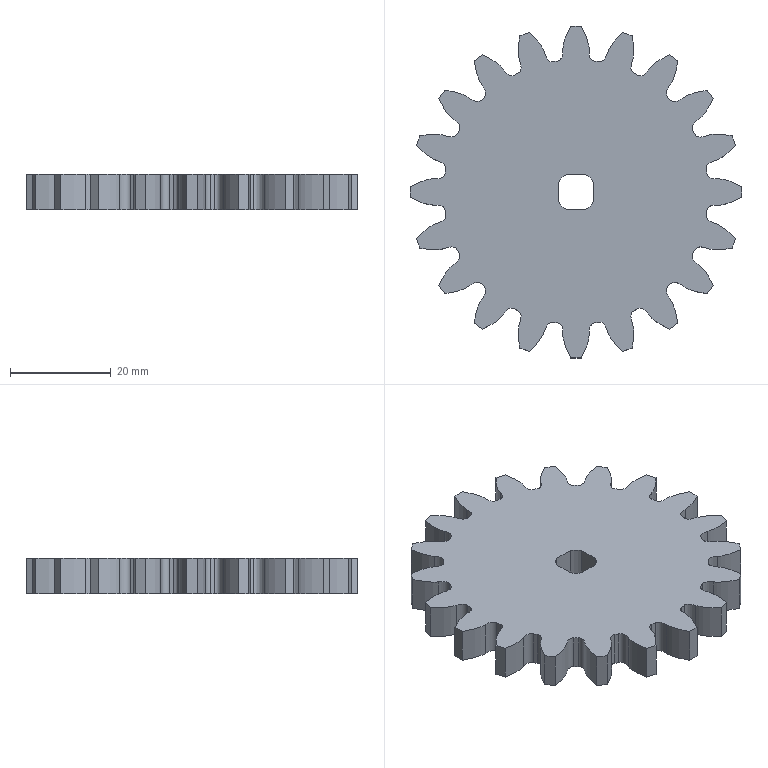Part | NX | features BREP 20, META 20, DATUM_CSYS 3, SKETCH 2, CYLINDER 1, EXTRUDE 1, FSET 1 | 1 solid | 130 faces | box 66 x 66 x 7 mm | volume 19139 mm3 | spline 100 | cylinder 24 | plane 6 | commonest cylinder face diameters 52.5 x20 8 x4